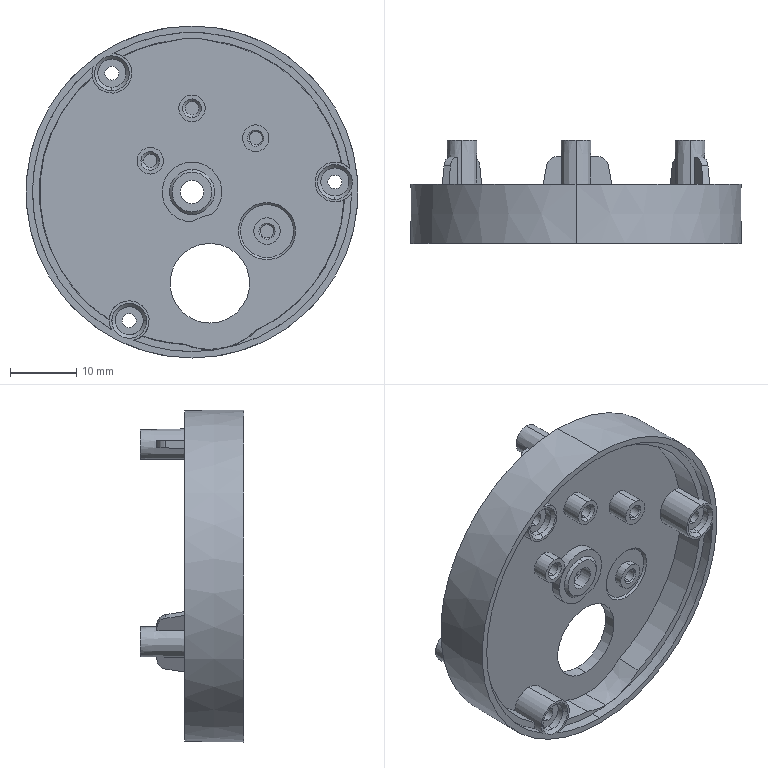Part | SolidWorks | features BaseBody 1 | 1 solid | 224 faces | box 50 x 15.55 x 50 mm | volume 5653 mm3 | plane 87 | cylinder 68 | cone 64 | spline 5 | commonest cylinder face diameters 4 x11 5.95 x11 2.02 x8 2 x6 2.1 x6 3.26 x6